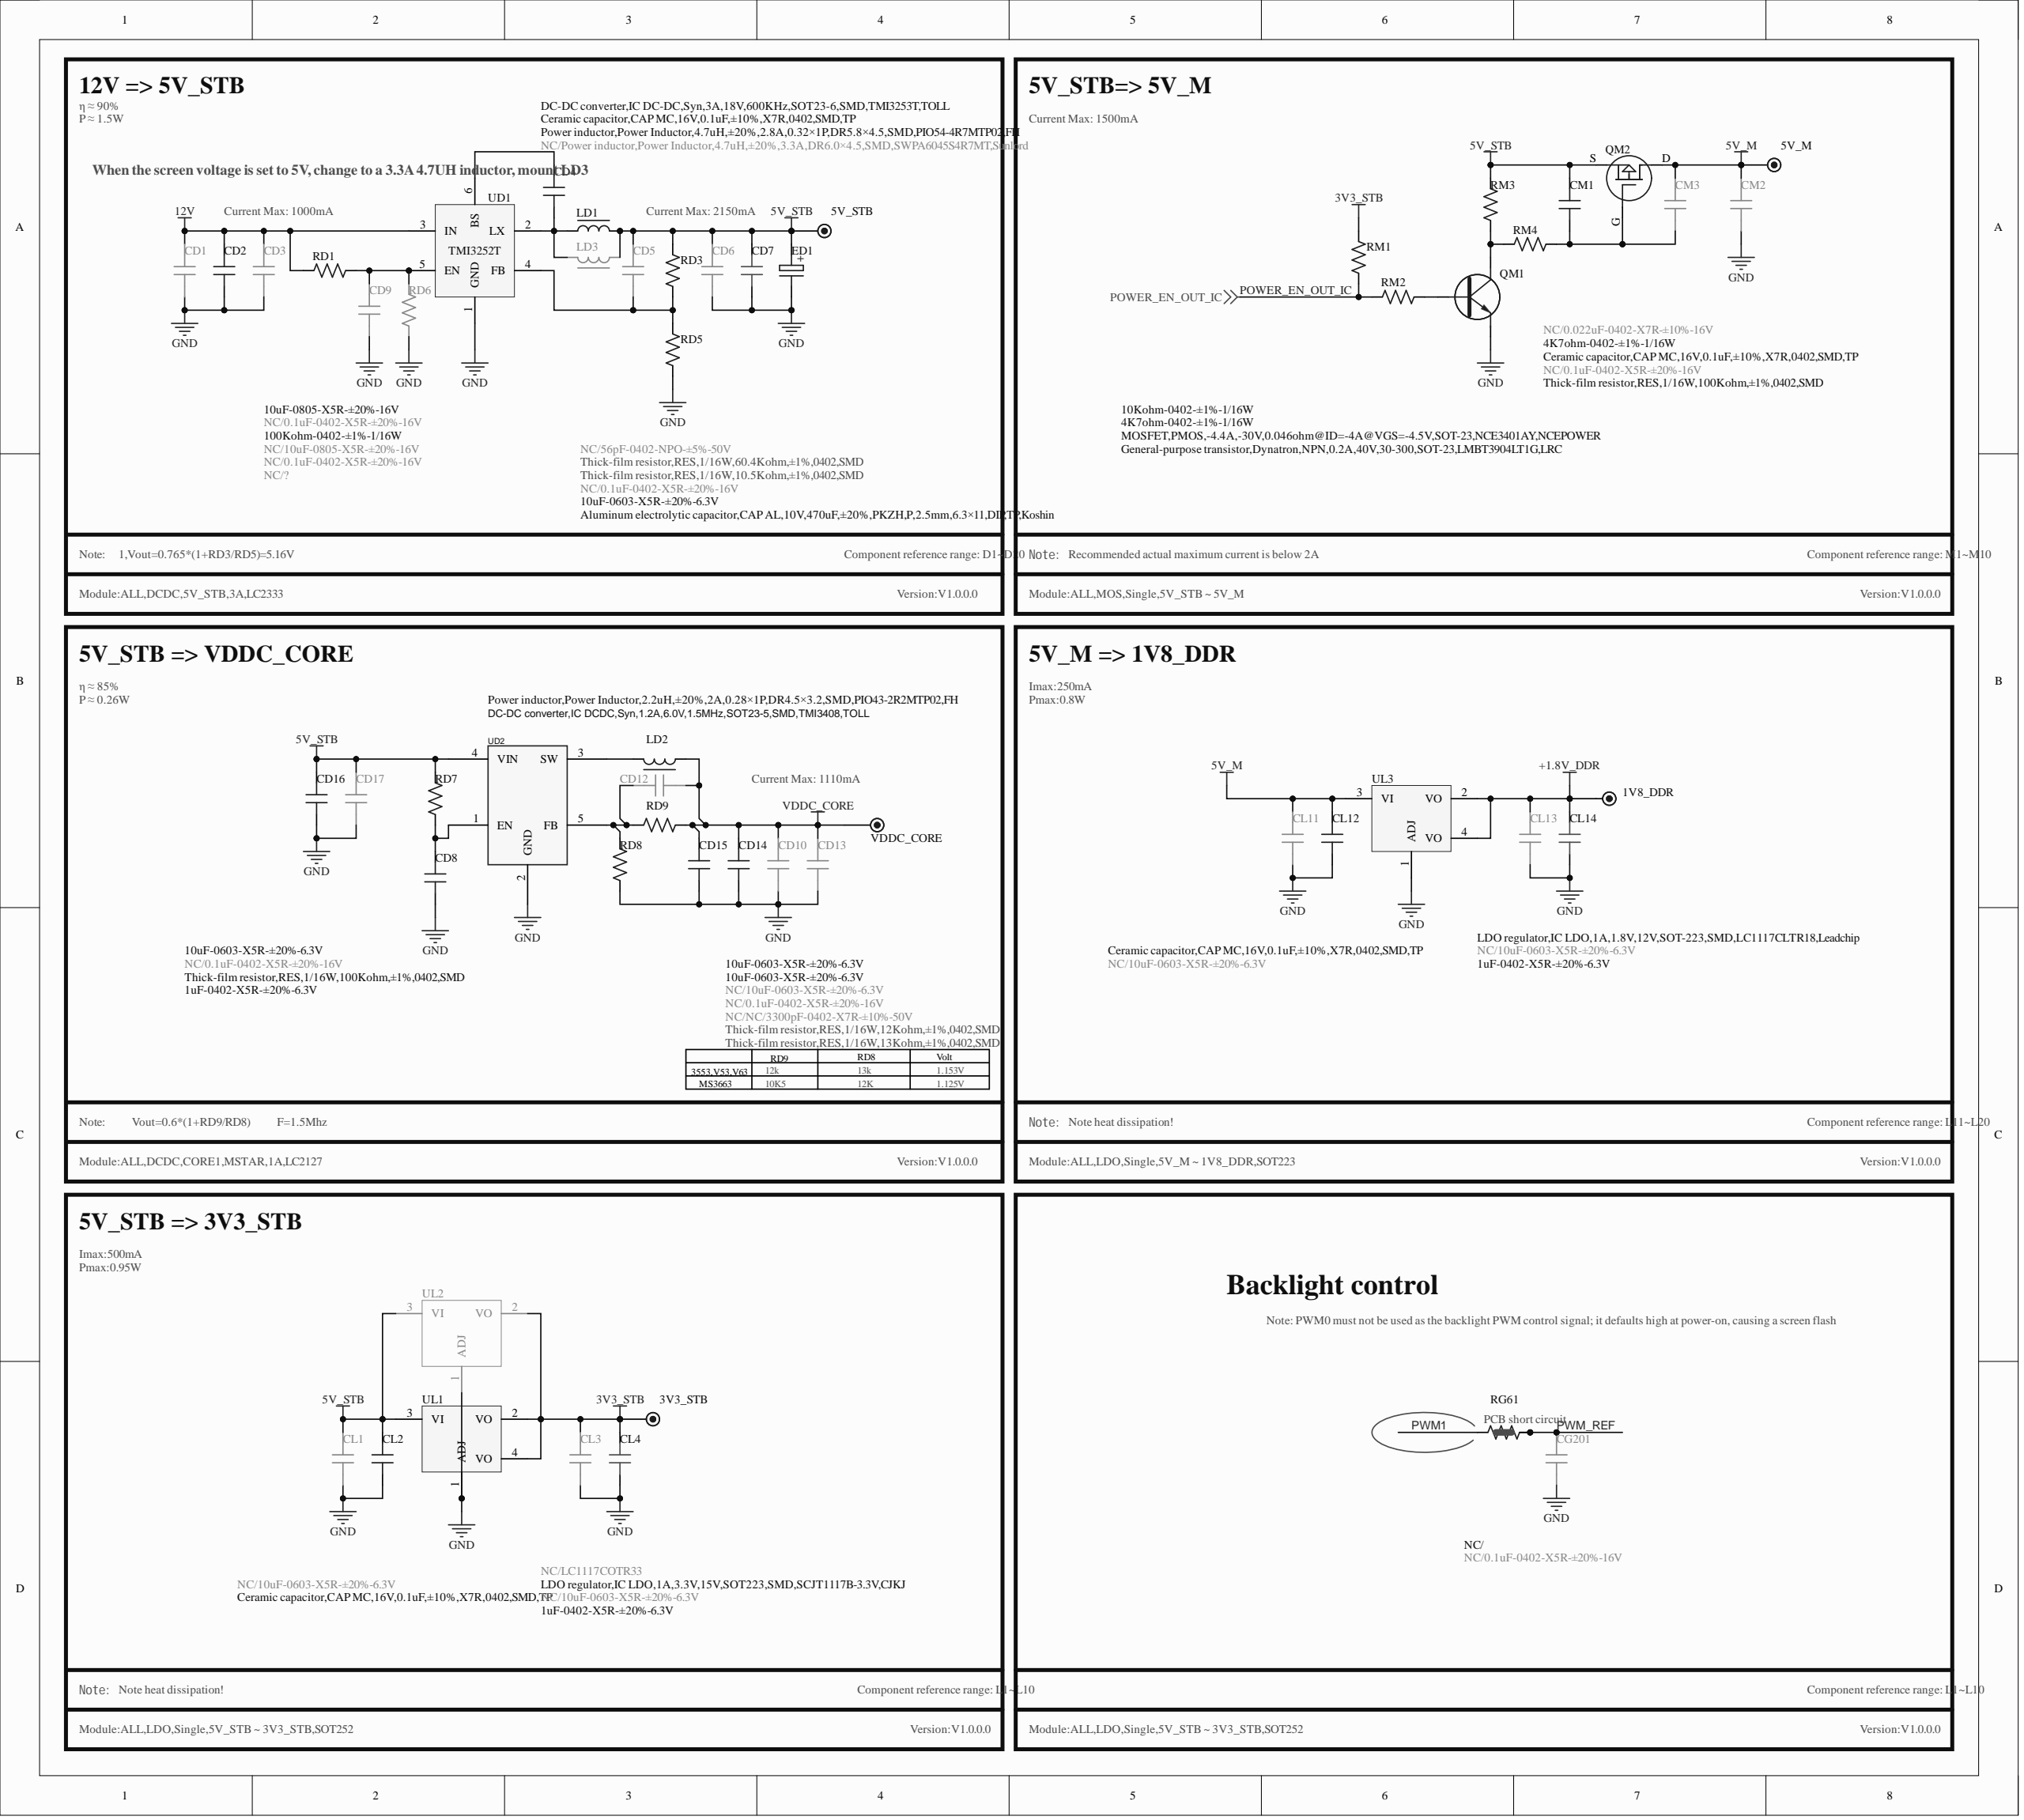Circuit board | Altium Designer | 527 parts | 243 nets | one sheet of the schematic
Parts on this sheet (reference | value | footprint):
1V8_DDR | TEST | TP
CD1 | NC/10uF-0805-X5R-±20%-16V | C0805
CD2 | 10uF-0805-X5R-±20%-16V | C0805
CD3 | NC/0.1uF-0402-X5R-±20%-16V | C0402
CD4 | Ceramic capacitor,CAP MC,16V,0.1uF,±10%,X7R,0402,SMD,TP | C0402
CD5 | NC/56pF-0402-NPO-±5%-50V | C0402
CD6 | NC/0.1uF-0402-X5R-±20%-16V | C0402
CD7 | 10uF-0603-X5R-±20%-6.3V | C0603
CD8 | 1uF-0402-X5R-±20%-6.3V | C0402
CD9 | NC/0.1uF-0402-X5R-±20%-16V | C0402
CD10 | NC/10uF-0603-X5R-±20%-6.3V | C0603
CD12 | NC/NC/3300pF-0402-X7R-±10%-50V | C0402
CD13 | NC/0.1uF-0402-X5R-±20%-16V | C0402
CD14 | 10uF-0603-X5R-±20%-6.3V | C0603
CD15 | 10uF-0603-X5R-±20%-6.3V | C0603
CD16 | 10uF-0603-X5R-±20%-6.3V | C0603
CD17 | NC/0.1uF-0402-X5R-±20%-16V | C0402
CG201 | NC/0.1uF-0402-X5R-±20%-16V | C0402
CL1 | NC/10uF-0603-X5R-±20%-6.3V | C0603
CL2 | Ceramic capacitor,CAP MC,16V,0.1uF,±10%,X7R,0402,SMD,TP | C0402
CL3 | NC/10uF-0603-X5R-±20%-6.3V | C0603
CL4 | 1uF-0402-X5R-±20%-6.3V | C0402
CL11 | NC/10uF-0603-X5R-±20%-6.3V | C0603
CL12 | Ceramic capacitor,CAP MC,16V,0.1uF,±10%,X7R,0402,SMD,TP | C0402
CL13 | NC/10uF-0603-X5R-±20%-6.3V | C0603
CL14 | 1uF-0402-X5R-±20%-6.3V | C0402
CM1 | Ceramic capacitor,CAP MC,16V,0.1uF,±10%,X7R,0402,SMD,TP | C0402
CM2 | NC/0.1uF-0402-X5R-±20%-16V | C0402
CM3 | NC/0.022uF-0402-X7R-±10%-16V | C0402
LD1 | Power inductor,Power Inductor,4.7uH,±20%,2.8A,0.32×1P,DR5.8×4.5,SMD,PIO54-4R7MTP02,FH | L(5.8*4.5)-S
LD2 | Power inductor,Power Inductor,2.2uH,±20%,2A,0.28×1P,DR4.5×3.2,SMD,PIO43-2R2MTP02,FH | L(4.5*3.5)-S
LD3 | NC/Power inductor,Power Inductor,4.7uH,±20%,3.3A,DR6.0×4.5,SMD,SWPA6045S4R7MT,Sunlord | L(6.0*4.5)-S
QM1 | General-purpose transistor,Dynatron,NPN,0.2A,40V,30-300,SOT-23,LMBT3904LT1G,LRC | SOT-23
QM2 | MOSFET,PMOS,-4.4A,-30V,0.046ohm@ID=-4A@VGS=-4.5V,SOT-23,NCE3401AY,NCEPOWER | SOT-23-1
RD1 | 100Kohm-0402-±1%-1/16W | R0402
RD3 | Thick-film resistor,RES,1/16W,60.4Kohm,±1%,0402,SMD | R0402
RD5 | Thick-film resistor,RES,1/16W,10.5Kohm,±1%,0402,SMD | R0402
RD6 | NC/? | R0402
RD7 | Thick-film resistor,RES,1/16W,100Kohm,±1%,0402,SMD | R0402
RD8 | Thick-film resistor,RES,1/16W,13Kohm,±1%,0402,SMD | R0402
RD9 | Thick-film resistor,RES,1/16W,12Kohm,±1%,0402,SMD | R0402
RG61 | NC/ | R0402SC
RM1 | 10Kohm-0402-±1%-1/16W | R0402
RM2 | 4K7ohm-0402-±1%-1/16W | R0402
RM3 | 4K7ohm-0402-±1%-1/16W | R0402
RM4 | Thick-film resistor,RES,1/16W,100Kohm,±1%,0402,SMD | R0402
UD1 | DC-DC converter,IC DC-DC,Syn,3A,18V,600KHz,SOT23-6,SMD,TMI3253T,TOLL | TSOT23-6
UD2 | DC-DC converter,IC DCDC,Syn,1.2A,6.0V,1.5MHz,SOT23-5,SMD,TMI3408,TOLL | SOT-23-5
UL1 | LDO regulator,IC LDO,1A,3.3V,15V,SOT223,SMD,SCJT1117B-3.3V,CJKJ | SOT-223
UL2 | NC/LC1117COTR33 | TO-252
UL3 | LDO regulator,IC LDO,1A,1.8V,12V,SOT-223,SMD,LC1117CLTR18,Leadchip | SOT-223
Nets of these parts (net: part-pin ...):
VDDC_CORE: CD10-2 CD12-2 CD13-2 CD14-2 CD15-2 LD2-1 RD9-1
PWM_REF: CG201-1 RG61-2 RG61-3
PWM1: RG61-1
POWER_EN_OUT_IC: RM1-1 RM2-1
NetQM1_C: QM1-C RM3-1 RM4-1
NetQM1_B: QM1-B RM2-2
NetLD2_2: LD2-2 UD2-3
NetCM1_1: CM1-1 CM3-2 QM2-G RM4-2
NetCD12_1: CD12-1 RD8-1 RD9-2 UD2-5
NetCD9_2: CD9-2 RD1-2 RD6-2 UD1-5
NetCD8_2: CD8-2 RD7-1 UD2-1
NetCD5_1: CD5-1 RD3-1 RD5-2 UD1-4
NetCD4_2: CD4-2 UD1-6
NetCD4_1: CD4-1 LD1-1 LD3-2 UD1-2
GND: CD1-2 CD2-2 CD3-1 CD6-1 CD7-1 CD8-1 CD9-1 CD10-1 CD13-1 CD14-1 CD15-1 CD16-1 CD17-1 CG201-2 CL1-1 CL2-1 CL3-1 CL4-1 CL11-1 CL12-1 CL13-1 CL14-1 CM2-1 QM1-E RD5-1 RD6-1 RD8-2 UD1-1 UD2-2 UL1-1 UL2-1 UL3-1
+1.8V_DDR: 1V8_DDR-1 CL13-2 CL14-2 UL3-2 UL3-4
12V: CD1-1 CD2-1 CD3-2 RD1-1 UD1-3
5V_STB: CD5-2 CD6-2 CD7-2 CD16-2 CD17-2 CL1-2 CL2-2 CM1-2 LD1-2 LD3-1 QM2-S RD3-2 RD7-2 RM3-2 UD2-4 UL1-3 UL2-3
5V_M: CL11-2 CL12-2 CM2-2 CM3-1 QM2-D UL3-3
3V3_STB: CL3-2 CL4-2 RM1-2 UL1-2 UL1-4 UL2-2